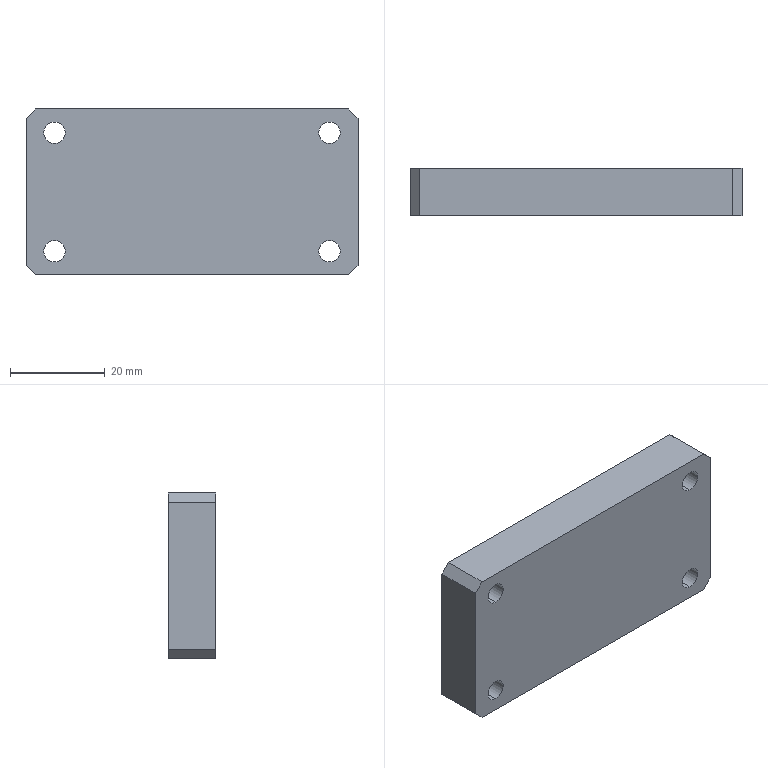Part | SolidWorks | features Chamfer 1, Extrusion 1, HoleWzd 1 | 1 solid | 30 faces | box 70 x 10 x 35 mm | volume 23097 mm3 | cylinder 16 | plane 14 | commonest cylinder face diameters 4.5 x8 8 x8
STEP:
#1=CARTESIAN_POINT('',(-29.,0.,-16.5));
#2=VERTEX_POINT('',#1);
#3=CARTESIAN_POINT('',(-29.,0.,-8.5));
#4=VERTEX_POINT('',#3);
#5=CARTESIAN_POINT('',(-29.,0.,-12.5));
#6=DIRECTION('',(0.,1.,0.));
#7=DIRECTION('',(0.,0.,1.));
#8=AXIS2_PLACEMENT_3D('',#5,#6,#7);
#9=CIRCLE('',#8,4.);
#10=EDGE_CURVE('',#2,#4,#9,.T.);
#11=ORIENTED_EDGE('',*,*,#10,.F.);
#12=CARTESIAN_POINT('',(-29.,5.,-16.5));
#13=VERTEX_POINT('',#12);
#14=CARTESIAN_POINT('',(-29.,5.,-16.5));
#15=DIRECTION('',(0.,1.,0.));
#16=VECTOR('',#15,1000.);
#17=LINE('',#14,#16);
#18=EDGE_CURVE('',#2,#13,#17,.T.);
#19=ORIENTED_EDGE('',*,*,#18,.T.);
#20=CARTESIAN_POINT('',(-29.,5.,-8.5));
#21=VERTEX_POINT('',#20);
#22=CARTESIAN_POINT('',(-29.,5.,-12.5));
#23=DIRECTION('',(0.,1.,0.));
#24=DIRECTION('',(0.,0.,1.));
#25=AXIS2_PLACEMENT_3D('',#22,#23,#24);
#26=CIRCLE('',#25,4.);
#27=EDGE_CURVE('',#13,#21,#26,.T.);
#28=ORIENTED_EDGE('',*,*,#27,.T.);
#29=CARTESIAN_POINT('',(-29.,5.,-8.5));
#30=DIRECTION('',(0.,1.,0.));
#31=VECTOR('',#30,1000.);
#32=LINE('',#29,#31);
#33=EDGE_CURVE('',#4,#21,#32,.T.);
#34=ORIENTED_EDGE('',*,*,#33,.F.);
#35=EDGE_LOOP('',(#11,#19,#28,#34));
#36=FACE_OUTER_BOUND('',#35,.T.);
#37=CARTESIAN_POINT('',(-29.,5.,-12.5));
#38=DIRECTION('',(0.,1.,0.));
#39=DIRECTION('',(0.,0.,1.));
#40=AXIS2_PLACEMENT_3D('',#37,#38,#39);
#41=CYLINDRICAL_SURFACE('',#40,4.);
#42=ADVANCED_FACE('',(#36),#41,.F.);
#43=CARTESIAN_POINT('',(-29.,-5.,-10.25));
#44=VERTEX_POINT('',#43);
#45=CARTESIAN_POINT('',(-29.,-5.,-14.75));
#46=VERTEX_POINT('',#45);
#47=CARTESIAN_POINT('',(-29.,-5.,-12.5));
#48=DIRECTION('',(0.,-1.,0.));
#49=DIRECTION('',(0.,0.,-1.));
#50=AXIS2_PLACEMENT_3D('',#47,#48,#49);
#51=CIRCLE('',#50,2.25);
#52=EDGE_CURVE('',#44,#46,#51,.T.);
#53=ORIENTED_EDGE('',*,*,#52,.T.);
#54=CARTESIAN_POINT('',(-29.,0.,-14.75));
#55=VERTEX_POINT('',#54);
#56=CARTESIAN_POINT('',(-29.,5.,-14.75));
#57=DIRECTION('',(0.,1.,0.));
#58=VECTOR('',#57,1000.);
#59=LINE('',#56,#58);
#60=EDGE_CURVE('',#46,#55,#59,.T.);
#61=ORIENTED_EDGE('',*,*,#60,.T.);
#62=CARTESIAN_POINT('',(-29.,0.,-10.25));
#63=VERTEX_POINT('',#62);
#64=CARTESIAN_POINT('',(-29.,0.,-12.5));
#65=DIRECTION('',(0.,1.,0.));
#66=DIRECTION('',(0.,0.,1.));
#67=AXIS2_PLACEMENT_3D('',#64,#65,#66);
#68=CIRCLE('',#67,2.25);
#69=EDGE_CURVE('',#55,#63,#68,.T.);
#70=ORIENTED_EDGE('',*,*,#69,.T.);
#71=CARTESIAN_POINT('',(-29.,5.,-10.25));
#72=DIRECTION('',(0.,1.,0.));
#73=VECTOR('',#72,1000.);
#74=LINE('',#71,#73);
#75=EDGE_CURVE('',#44,#63,#74,.T.);
#76=ORIENTED_EDGE('',*,*,#75,.F.);
#77=EDGE_LOOP('',(#53,#61,#70,#76));
#78=FACE_OUTER_BOUND('',#77,.T.);
#79=CARTESIAN_POINT('',(-29.,5.,-12.5));
#80=DIRECTION('',(0.,1.,0.));
#81=DIRECTION('',(0.,0.,1.));
#82=AXIS2_PLACEMENT_3D('',#79,#80,#81);
#83=CYLINDRICAL_SURFACE('',#82,2.25);
#84=ADVANCED_FACE('',(#78),#83,.F.);
#85=CARTESIAN_POINT('',(-29.,0.,8.5));
#86=VERTEX_POINT('',#85);
#87=CARTESIAN_POINT('',(-29.,0.,16.5));
#88=VERTEX_POINT('',#87);
#89=CARTESIAN_POINT('',(-29.,0.,12.5));
#90=DIRECTION('',(0.,1.,0.));
#91=DIRECTION('',(0.,0.,1.));
#92=AXIS2_PLACEMENT_3D('',#89,#90,#91);
#93=CIRCLE('',#92,4.);
#94=EDGE_CURVE('',#86,#88,#93,.T.);
#95=ORIENTED_EDGE('',*,*,#94,.F.);
#96=CARTESIAN_POINT('',(-29.,5.,8.5));
#97=VERTEX_POINT('',#96);
#98=CARTESIAN_POINT('',(-29.,5.,8.5));
#99=DIRECTION('',(0.,1.,0.));
#100=VECTOR('',#99,1000.);
#101=LINE('',#98,#100);
#102=EDGE_CURVE('',#86,#97,#101,.T.);
#103=ORIENTED_EDGE('',*,*,#102,.T.);
#104=CARTESIAN_POINT('',(-29.,5.,16.5));
#105=VERTEX_POINT('',#104);
#106=CARTESIAN_POINT('',(-29.,5.,12.5));
#107=DIRECTION('',(0.,1.,0.));
#108=DIRECTION('',(0.,0.,1.));
#109=AXIS2_PLACEMENT_3D('',#106,#107,#108);
#110=CIRCLE('',#109,4.);
#111=EDGE_CURVE('',#97,#105,#110,.T.);
#112=ORIENTED_EDGE('',*,*,#111,.T.);
#113=CARTESIAN_POINT('',(-29.,5.,16.5));
#114=DIRECTION('',(0.,1.,0.));
#115=VECTOR('',#114,1000.);
#116=LINE('',#113,#115);
#117=EDGE_CURVE('',#88,#105,#116,.T.);
#118=ORIENTED_EDGE('',*,*,#117,.F.);
#119=EDGE_LOOP('',(#95,#103,#112,#118));
#120=FACE_OUTER_BOUND('',#119,.T.);
#121=CARTESIAN_POINT('',(-29.,5.,12.5));
#122=DIRECTION('',(0.,1.,0.));
#123=DIRECTION('',(0.,0.,1.));
#124=AXIS2_PLACEMENT_3D('',#121,#122,#123);
#125=CYLINDRICAL_SURFACE('',#124,4.);
#126=ADVANCED_FACE('',(#120),#125,.F.);
#127=CARTESIAN_POINT('',(-29.,-5.,14.75));
#128=VERTEX_POINT('',#127);
#129=CARTESIAN_POINT('',(-29.,-5.,10.25));
#130=VERTEX_POINT('',#129);
#131=CARTESIAN_POINT('',(-29.,-5.,12.5));
#132=DIRECTION('',(0.,-1.,0.));
#133=DIRECTION('',(0.,0.,-1.));
#134=AXIS2_PLACEMENT_3D('',#131,#132,#133);
#135=CIRCLE('',#134,2.25);
#136=EDGE_CURVE('',#128,#130,#135,.T.);
#137=ORIENTED_EDGE('',*,*,#136,.T.);
#138=CARTESIAN_POINT('',(-29.,0.,10.25));
#139=VERTEX_POINT('',#138);
#140=CARTESIAN_POINT('',(-29.,5.,10.25));
#141=DIRECTION('',(0.,1.,0.));
#142=VECTOR('',#141,1000.);
#143=LINE('',#140,#142);
#144=EDGE_CURVE('',#130,#139,#143,.T.);
#145=ORIENTED_EDGE('',*,*,#144,.T.);
#146=CARTESIAN_POINT('',(-29.,0.,14.75));
#147=VERTEX_POINT('',#146);
#148=CARTESIAN_POINT('',(-29.,0.,12.5));
#149=DIRECTION('',(0.,1.,0.));
#150=DIRECTION('',(0.,0.,1.));
#151=AXIS2_PLACEMENT_3D('',#148,#149,#150);
#152=CIRCLE('',#151,2.25);
#153=EDGE_CURVE('',#139,#147,#152,.T.);
#154=ORIENTED_EDGE('',*,*,#153,.T.);
#155=CARTESIAN_POINT('',(-29.,5.,14.75));
#156=DIRECTION('',(0.,1.,0.));
#157=VECTOR('',#156,1000.);
#158=LINE('',#155,#157);
#159=EDGE_CURVE('',#128,#147,#158,.T.);
#160=ORIENTED_EDGE('',*,*,#159,.F.);
#161=EDGE_LOOP('',(#137,#145,#154,#160));
#162=FACE_OUTER_BOUND('',#161,.T.);
#163=CARTESIAN_POINT('',(-29.,5.,12.5));
#164=DIRECTION('',(0.,1.,0.));
#165=DIRECTION('',(0.,0.,1.));
#166=AXIS2_PLACEMENT_3D('',#163,#164,#165);
#167=CYLINDRICAL_SURFACE('',#166,2.25);
#168=ADVANCED_FACE('',(#162),#167,.F.);
#169=CARTESIAN_POINT('',(29.,0.,-16.5));
#170=VERTEX_POINT('',#169);
#171=CARTESIAN_POINT('',(29.,0.,-8.5));
#172=VERTEX_POINT('',#171);
#173=CARTESIAN_POINT('',(29.,0.,-12.5));
#174=DIRECTION('',(0.,1.,0.));
#175=DIRECTION('',(0.,0.,1.));
#176=AXIS2_PLACEMENT_3D('',#173,#174,#175);
#177=CIRCLE('',#176,4.);
#178=EDGE_CURVE('',#170,#172,#177,.T.);
#179=ORIENTED_EDGE('',*,*,#178,.F.);
#180=CARTESIAN_POINT('',(29.,5.,-16.5));
#181=VERTEX_POINT('',#180);
#182=CARTESIAN_POINT('',(29.,5.,-16.5));
#183=DIRECTION('',(0.,1.,0.));
#184=VECTOR('',#183,1000.);
#185=LINE('',#182,#184);
#186=EDGE_CURVE('',#170,#181,#185,.T.);
#187=ORIENTED_EDGE('',*,*,#186,.T.);
#188=CARTESIAN_POINT('',(29.,5.,-8.5));
#189=VERTEX_POINT('',#188);
#190=CARTESIAN_POINT('',(29.,5.,-12.5));
#191=DIRECTION('',(0.,1.,0.));
#192=DIRECTION('',(0.,0.,1.));
#193=AXIS2_PLACEMENT_3D('',#190,#191,#192);
#194=CIRCLE('',#193,4.);
#195=EDGE_CURVE('',#181,#189,#194,.T.);
#196=ORIENTED_EDGE('',*,*,#195,.T.);
#197=CARTESIAN_POINT('',(29.,5.,-8.5));
#198=DIRECTION('',(0.,1.,0.));
#199=VECTOR('',#198,1000.);
#200=LINE('',#197,#199);
#201=EDGE_CURVE('',#172,#189,#200,.T.);
#202=ORIENTED_EDGE('',*,*,#201,.F.);
#203=EDGE_LOOP('',(#179,#187,#196,#202));
#204=FACE_OUTER_BOUND('',#203,.T.);
#205=CARTESIAN_POINT('',(29.,5.,-12.5));
#206=DIRECTION('',(0.,1.,0.));
#207=DIRECTION('',(0.,0.,1.));
#208=AXIS2_PLACEMENT_3D('',#205,#206,#207);
#209=CYLINDRICAL_SURFACE('',#208,4.);
#210=ADVANCED_FACE('',(#204),#209,.F.);
#211=CARTESIAN_POINT('',(29.,-5.,-10.25));
#212=VERTEX_POINT('',#211);
#213=CARTESIAN_POINT('',(29.,-5.,-14.75));
#214=VERTEX_POINT('',#213);
#215=CARTESIAN_POINT('',(29.,-5.,-12.5));
#216=DIRECTION('',(0.,-1.,0.));
#217=DIRECTION('',(0.,0.,-1.));
#218=AXIS2_PLACEMENT_3D('',#215,#216,#217);
#219=CIRCLE('',#218,2.25);
#220=EDGE_CURVE('',#212,#214,#219,.T.);
#221=ORIENTED_EDGE('',*,*,#220,.T.);
#222=CARTESIAN_POINT('',(29.,0.,-14.75));
#223=VERTEX_POINT('',#222);
#224=CARTESIAN_POINT('',(29.,5.,-14.75));
#225=DIRECTION('',(0.,1.,0.));
#226=VECTOR('',#225,1000.);
#227=LINE('',#224,#226);
#228=EDGE_CURVE('',#214,#223,#227,.T.);
#229=ORIENTED_EDGE('',*,*,#228,.T.);
#230=CARTESIAN_POINT('',(29.,0.,-10.25));
#231=VERTEX_POINT('',#230);
#232=CARTESIAN_POINT('',(29.,0.,-12.5));
#233=DIRECTION('',(0.,1.,0.));
#234=DIRECTION('',(0.,0.,1.));
#235=AXIS2_PLACEMENT_3D('',#232,#233,#234);
#236=CIRCLE('',#235,2.25);
#237=EDGE_CURVE('',#223,#231,#236,.T.);
#238=ORIENTED_EDGE('',*,*,#237,.T.);
#239=CARTESIAN_POINT('',(29.,5.,-10.25));
#240=DIRECTION('',(0.,1.,0.));
#241=VECTOR('',#240,1000.);
#242=LINE('',#239,#241);
#243=EDGE_CURVE('',#212,#231,#242,.T.);
#244=ORIENTED_EDGE('',*,*,#243,.F.);
#245=EDGE_LOOP('',(#221,#229,#238,#244));
#246=FACE_OUTER_BOUND('',#245,.T.);
#247=CARTESIAN_POINT('',(29.,5.,-12.5));
#248=DIRECTION('',(0.,1.,0.));
#249=DIRECTION('',(0.,0.,1.));
#250=AXIS2_PLACEMENT_3D('',#247,#248,#249);
#251=CYLINDRICAL_SURFACE('',#250,2.25);
#252=ADVANCED_FACE('',(#246),#251,.F.);
#253=CARTESIAN_POINT('',(29.,0.,8.5));
#254=VERTEX_POINT('',#253);
#255=CARTESIAN_POINT('',(29.,0.,16.5));
#256=VERTEX_POINT('',#255);
#257=CARTESIAN_POINT('',(29.,0.,12.5));
#258=DIRECTION('',(0.,1.,0.));
#259=DIRECTION('',(0.,0.,1.));
#260=AXIS2_PLACEMENT_3D('',#257,#258,#259);
#261=CIRCLE('',#260,4.);
#262=EDGE_CURVE('',#254,#256,#261,.T.);
#263=ORIENTED_EDGE('',*,*,#262,.F.);
#264=CARTESIAN_POINT('',(29.,5.,8.5));
#265=VERTEX_POINT('',#264);
#266=CARTESIAN_POINT('',(29.,5.,8.5));
#267=DIRECTION('',(0.,1.,0.));
#268=VECTOR('',#267,1000.);
#269=LINE('',#266,#268);
#270=EDGE_CURVE('',#254,#265,#269,.T.);
#271=ORIENTED_EDGE('',*,*,#270,.T.);
#272=CARTESIAN_POINT('',(29.,5.,16.5));
#273=VERTEX_POINT('',#272);
#274=CARTESIAN_POINT('',(29.,5.,12.5));
#275=DIRECTION('',(0.,1.,0.));
#276=DIRECTION('',(0.,0.,1.));
#277=AXIS2_PLACEMENT_3D('',#274,#275,#276);
#278=CIRCLE('',#277,4.);
#279=EDGE_CURVE('',#265,#273,#278,.T.);
#280=ORIENTED_EDGE('',*,*,#279,.T.);
#281=CARTESIAN_POINT('',(29.,5.,16.5));
#282=DIRECTION('',(0.,1.,0.));
#283=VECTOR('',#282,1000.);
#284=LINE('',#281,#283);
#285=EDGE_CURVE('',#256,#273,#284,.T.);
#286=ORIENTED_EDGE('',*,*,#285,.F.);
#287=EDGE_LOOP('',(#263,#271,#280,#286));
#288=FACE_OUTER_BOUND('',#287,.T.);
#289=CARTESIAN_POINT('',(29.,5.,12.5));
#290=DIRECTION('',(0.,1.,0.));
#291=DIRECTION('',(0.,0.,1.));
#292=AXIS2_PLACEMENT_3D('',#289,#290,#291);
#293=CYLINDRICAL_SURFACE('',#292,4.);
#294=ADVANCED_FACE('',(#288),#293,.F.);
#295=CARTESIAN_POINT('',(29.,-5.,14.75));
#296=VERTEX_POINT('',#295);
#297=CARTESIAN_POINT('',(29.,-5.,10.25));
#298=VERTEX_POINT('',#297);
#299=CARTESIAN_POINT('',(29.,-5.,12.5));
#300=DIRECTION('',(0.,-1.,0.));
#301=DIRECTION('',(0.,0.,-1.));
#302=AXIS2_PLACEMENT_3D('',#299,#300,#301);
#303=CIRCLE('',#302,2.25);
#304=EDGE_CURVE('',#296,#298,#303,.T.);
#305=ORIENTED_EDGE('',*,*,#304,.T.);
#306=CARTESIAN_POINT('',(29.,0.,10.25));
#307=VERTEX_POINT('',#306);
#308=CARTESIAN_POINT('',(29.,5.,10.25));
#309=DIRECTION('',(0.,1.,0.));
#310=VECTOR('',#309,1000.);
#311=LINE('',#308,#310);
#312=EDGE_CURVE('',#298,#307,#311,.T.);
#313=ORIENTED_EDGE('',*,*,#312,.T.);
#314=CARTESIAN_POINT('',(29.,0.,14.75));
#315=VERTEX_POINT('',#314);
#316=CARTESIAN_POINT('',(29.,0.,12.5));
#317=DIRECTION('',(0.,1.,0.));
#318=DIRECTION('',(0.,0.,1.));
#319=AXIS2_PLACEMENT_3D('',#316,#317,#318);
#320=CIRCLE('',#319,2.25);
#321=EDGE_CURVE('',#307,#315,#320,.T.);
#322=ORIENTED_EDGE('',*,*,#321,.T.);
#323=CARTESIAN_POINT('',(29.,5.,14.75));
#324=DIRECTION('',(0.,1.,0.));
#325=VECTOR('',#324,1000.);
#326=LINE('',#323,#325);
#327=EDGE_CURVE('',#296,#315,#326,.T.);
#328=ORIENTED_EDGE('',*,*,#327,.F.);
#329=EDGE_LOOP('',(#305,#313,#322,#328));
#330=FACE_OUTER_BOUND('',#329,.T.);
#331=CARTESIAN_POINT('',(29.,5.,12.5));
#332=DIRECTION('',(0.,1.,0.));
#333=DIRECTION('',(0.,0.,1.));
#334=AXIS2_PLACEMENT_3D('',#331,#332,#333);
#335=CYLINDRICAL_SURFACE('',#334,2.25);
#336=ADVANCED_FACE('',(#330),#335,.F.);
#337=CARTESIAN_POINT('',(-29.,5.,-12.5));
#338=DIRECTION('',(0.,1.,0.));
#339=DIRECTION('',(0.,0.,1.));
#340=AXIS2_PLACEMENT_3D('',#337,#338,#339);
#341=CIRCLE('',#340,4.);
#342=EDGE_CURVE('',#21,#13,#341,.T.);
#343=ORIENTED_EDGE('',*,*,#342,.F.);
#344=ORIENTED_EDGE('',*,*,#27,.F.);
#345=EDGE_LOOP('',(#343,#344));
#346=FACE_BOUND('',#345,.T.);
#347=CARTESIAN_POINT('',(29.,5.,12.5));
#348=DIRECTION('',(0.,1.,0.));
#349=DIRECTION('',(0.,0.,1.));
#350=AXIS2_PLACEMENT_3D('',#347,#348,#349);
#351=CIRCLE('',#350,4.);
#352=EDGE_CURVE('',#273,#265,#351,.T.);
#353=ORIENTED_EDGE('',*,*,#352,.F.);
#354=ORIENTED_EDGE('',*,*,#279,.F.);
#355=EDGE_LOOP('',(#353,#354));
#356=FACE_BOUND('',#355,.T.);
#357=CARTESIAN_POINT('',(33.,5.,-17.5));
#358=VERTEX_POINT('',#357);
#359=CARTESIAN_POINT('',(-33.,5.,-17.5));
#360=VERTEX_POINT('',#359);
#361=CARTESIAN_POINT('',(-35.,5.,-17.5));
#362=DIRECTION('',(-1.,0.,0.));
#363=VECTOR('',#362,1000.);
#364=LINE('',#361,#363);
#365=EDGE_CURVE('',#358,#360,#364,.T.);
#366=ORIENTED_EDGE('',*,*,#365,.T.);
#367=CARTESIAN_POINT('',(-35.,5.,-15.5));
#368=VERTEX_POINT('',#367);
#369=CARTESIAN_POINT('',(-35.,5.,-15.5));
#370=DIRECTION('',(-0.7071,0.,0.7071));
#371=VECTOR('',#370,1000.);
#372=LINE('',#369,#371);
#373=EDGE_CURVE('',#360,#368,#372,.T.);
#374=ORIENTED_EDGE('',*,*,#373,.T.);
#375=CARTESIAN_POINT('',(-35.,5.,15.5));
#376=VERTEX_POINT('',#375);
#377=CARTESIAN_POINT('',(-35.,5.,17.5));
#378=DIRECTION('',(0.,0.,1.));
#379=VECTOR('',#378,1000.);
#380=LINE('',#377,#379);
#381=EDGE_CURVE('',#368,#376,#380,.T.);
#382=ORIENTED_EDGE('',*,*,#381,.T.);
#383=CARTESIAN_POINT('',(-33.,5.,17.5));
#384=VERTEX_POINT('',#383);
#385=CARTESIAN_POINT('',(-33.,5.,17.5));
#386=DIRECTION('',(0.7071,0.,0.7071));
#387=VECTOR('',#386,1000.);
#388=LINE('',#385,#387);
#389=EDGE_CURVE('',#376,#384,#388,.T.);
#390=ORIENTED_EDGE('',*,*,#389,.T.);
#391=CARTESIAN_POINT('',(33.,5.,17.5));
#392=VERTEX_POINT('',#391);
#393=CARTESIAN_POINT('',(-35.,5.,17.5));
#394=DIRECTION('',(1.,0.,0.));
#395=VECTOR('',#394,1000.);
#396=LINE('',#393,#395);
#397=EDGE_CURVE('',#384,#392,#396,.T.);
#398=ORIENTED_EDGE('',*,*,#397,.T.);
#399=CARTESIAN_POINT('',(35.,5.,15.5));
#400=VERTEX_POINT('',#399);
#401=CARTESIAN_POINT('',(35.,5.,15.5));
#402=DIRECTION('',(0.7071,0.,-0.7071));
#403=VECTOR('',#402,1000.);
#404=LINE('',#401,#403);
#405=EDGE_CURVE('',#392,#400,#404,.T.);
#406=ORIENTED_EDGE('',*,*,#405,.T.);
#407=CARTESIAN_POINT('',(35.,5.,-15.5));
#408=VERTEX_POINT('',#407);
#409=CARTESIAN_POINT('',(35.,5.,17.5));
#410=DIRECTION('',(0.,0.,-1.));
#411=VECTOR('',#410,1000.);
#412=LINE('',#409,#411);
#413=EDGE_CURVE('',#400,#408,#412,.T.);
#414=ORIENTED_EDGE('',*,*,#413,.T.);
#415=CARTESIAN_POINT('',(33.,5.,-17.5));
#416=DIRECTION('',(-0.7071,0.,-0.7071));
#417=VECTOR('',#416,1000.);
#418=LINE('',#415,#417);
#419=EDGE_CURVE('',#408,#358,#418,.T.);
#420=ORIENTED_EDGE('',*,*,#419,.T.);
#421=EDGE_LOOP('',(#366,#374,#382,#390,#398,#406,#414,#420));
#422=FACE_OUTER_BOUND('',#421,.T.);
#423=CARTESIAN_POINT('',(29.,5.,-12.5));
#424=DIRECTION('',(0.,1.,0.));
#425=DIRECTION('',(0.,0.,1.));
#426=AXIS2_PLACEMENT_3D('',#423,#424,#425);
#427=CIRCLE('',#426,4.);
#428=EDGE_CURVE('',#189,#181,#427,.T.);
#429=ORIENTED_EDGE('',*,*,#428,.F.);
#430=ORIENTED_EDGE('',*,*,#195,.F.);
#431=EDGE_LOOP('',(#429,#430));
#432=FACE_BOUND('',#431,.T.);
#433=CARTESIAN_POINT('',(-29.,5.,12.5));
#434=DIRECTION('',(0.,1.,0.));
#435=DIRECTION('',(0.,0.,1.));
#436=AXIS2_PLACEMENT_3D('',#433,#434,#435);
#437=CIRCLE('',#436,4.);
#438=EDGE_CURVE('',#105,#97,#437,.T.);
#439=ORIENTED_EDGE('',*,*,#438,.F.);
#440=ORIENTED_EDGE('',*,*,#111,.F.);
#441=EDGE_LOOP('',(#439,#440));
#442=FACE_BOUND('',#441,.T.);
#443=CARTESIAN_POINT('',(0.,5.,0.));
#444=DIRECTION('',(0.,-1.,0.));
#445=DIRECTION('',(0.,0.,-1.));
#446=AXIS2_PLACEMENT_3D('',#443,#444,#445);
#447=PLANE('',#446);
#448=ADVANCED_FACE('',(#346,#356,#422,#432,#442),#447,.F.);
#449=CARTESIAN_POINT('',(35.,-5.,15.5));
#450=VERTEX_POINT('',#449);
#451=CARTESIAN_POINT('',(35.,-5.,-15.5));
#452=VERTEX_POINT('',#451);
#453=CARTESIAN_POINT('',(35.,-5.,17.5));
#454=DIRECTION('',(0.,0.,-1.));
#455=VECTOR('',#454,1000.);
#456=LINE('',#453,#455);
#457=EDGE_CURVE('',#450,#452,#456,.T.);
#458=ORIENTED_EDGE('',*,*,#457,.T.);
#459=CARTESIAN_POINT('',(35.,5.,-15.5));
#460=DIRECTION('',(0.,1.,0.));
#461=VECTOR('',#460,1000.);
#462=LINE('',#459,#461);
#463=EDGE_CURVE('',#452,#408,#462,.T.);
#464=ORIENTED_EDGE('',*,*,#463,.T.);
#465=ORIENTED_EDGE('',*,*,#413,.F.);
#466=CARTESIAN_POINT('',(35.,5.,15.5));
#467=DIRECTION('',(0.,-1.,0.));
#468=VECTOR('',#467,1000.);
#469=LINE('',#466,#468);
#470=EDGE_CURVE('',#400,#450,#469,.T.);
#471=ORIENTED_EDGE('',*,*,#470,.T.);
#472=EDGE_LOOP('',(#458,#464,#465,#471));
#473=FACE_OUTER_BOUND('',#472,.T.);
#474=CARTESIAN_POINT('',(35.,5.,17.5));
#475=DIRECTION('',(-1.,0.,0.));
#476=DIRECTION('',(0.,0.,1.));
#477=AXIS2_PLACEMENT_3D('',#474,#475,#476);
#478=PLANE('',#477);
#479=ADVANCED_FACE('',(#473),#478,.F.);
#480=CARTESIAN_POINT('',(33.,-5.,-17.5));
#481=VERTEX_POINT('',#480);
#482=CARTESIAN_POINT('',(-33.,-5.,-17.5));
#483=VERTEX_POINT('',#482);
#484=CARTESIAN_POINT('',(-35.,-5.,-17.5));
#485=DIRECTION('',(-1.,0.,0.));
#486=VECTOR('',#485,1000.);
#487=LINE('',#484,#486);
#488=EDGE_CURVE('',#481,#483,#487,.T.);
#489=ORIENTED_EDGE('',*,*,#488,.T.);
#490=CARTESIAN_POINT('',(-33.,5.,-17.5));
#491=DIRECTION('',(0.,1.,0.));
#492=VECTOR('',#491,1000.);
#493=LINE('',#490,#492);
#494=EDGE_CURVE('',#483,#360,#493,.T.);
#495=ORIENTED_EDGE('',*,*,#494,.T.);
#496=ORIENTED_EDGE('',*,*,#365,.F.);
#497=CARTESIAN_POINT('',(33.,5.,-17.5));
#498=DIRECTION('',(0.,-1.,0.));
#499=VECTOR('',#498,1000.);
#500=LINE('',#497,#499);
#501=EDGE_CURVE('',#358,#481,#500,.T.);
#502=ORIENTED_EDGE('',*,*,#501,.T.);
#503=EDGE_LOOP('',(#489,#495,#496,#502));
#504=FACE_OUTER_BOUND('',#503,.T.);
#505=CARTESIAN_POINT('',(-35.,5.,-17.5));
#506=DIRECTION('',(0.,0.,1.));
#507=DIRECTION('',(1.,0.,0.));
#508=AXIS2_PLACEMENT_3D('',#505,#506,#507);
#509=PLANE('',#508);
#510=ADVANCED_FACE('',(#504),#509,.F.);
#511=ORIENTED_EDGE('',*,*,#381,.F.);
#512=CARTESIAN_POINT('',(-35.,-5.,-15.5));
#513=VERTEX_POINT('',#512);
#514=CARTESIAN_POINT('',(-35.,5.,-15.5));
#515=DIRECTION('',(0.,-1.,0.));
#516=VECTOR('',#515,1000.);
#517=LINE('',#514,#516);
#518=EDGE_CURVE('',#368,#513,#517,.T.);
#519=ORIENTED_EDGE('',*,*,#518,.T.);
#520=CARTESIAN_POINT('',(-35.,-5.,15.5));
#521=VERTEX_POINT('',#520);
#522=CARTESIAN_POINT('',(-35.,-5.,17.5));
#523=DIRECTION('',(0.,0.,1.));
#524=VECTOR('',#523,1000.);
#525=LINE('',#522,#524);
#526=EDGE_CURVE('',#513,#521,#525,.T.);
#527=ORIENTED_EDGE('',*,*,#526,.T.);
#528=CARTESIAN_POINT('',(-35.,5.,15.5));
#529=DIRECTION('',(0.,1.,0.));
#530=VECTOR('',#529,1000.);
#531=LINE('',#528,#530);
#532=EDGE_CURVE('',#521,#376,#531,.T.);
#533=ORIENTED_EDGE('',*,*,#532,.T.);
#534=EDGE_LOOP('',(#511,#519,#527,#533));
#535=FACE_OUTER_BOUND('',#534,.T.);
#536=CARTESIAN_POINT('',(-35.,5.,17.5));
#537=DIRECTION('',(1.,0.,0.));
#538=DIRECTION('',(0.,0.,-1.));
#539=AXIS2_PLACEMENT_3D('',#536,#537,#538);
#540=PLANE('',#539);
#541=ADVANCED_FACE('',(#535),#540,.F.);
#542=CARTESIAN_POINT('',(-33.,-5.,17.5));
#543=VERTEX_POINT('',#542);
#544=CARTESIAN_POINT('',(33.,-5.,17.5));
#545=VERTEX_POINT('',#544);
#546=CARTESIAN_POINT('',(-35.,-5.,17.5));
#547=DIRECTION('',(1.,0.,0.));
#548=VECTOR('',#547,1000.);
#549=LINE('',#546,#548);
#550=EDGE_CURVE('',#543,#545,#549,.T.);
#551=ORIENTED_EDGE('',*,*,#550,.T.);
#552=CARTESIAN_POINT('',(33.,5.,17.5));
#553=DIRECTION('',(0.,1.,0.));
#554=VECTOR('',#553,1000.);
#555=LINE('',#552,#554);
#556=EDGE_CURVE('',#545,#392,#555,.T.);
#557=ORIENTED_EDGE('',*,*,#556,.T.);
#558=ORIENTED_EDGE('',*,*,#397,.F.);
#559=CARTESIAN_POINT('',(-33.,5.,17.5));
#560=DIRECTION('',(0.,-1.,0.));
#561=VECTOR('',#560,1000.);
#562=LINE('',#559,#561);
#563=EDGE_CURVE('',#384,#543,#562,.T.);
#564=ORIENTED_EDGE('',*,*,#563,.T.);
#565=EDGE_LOOP('',(#551,#557,#558,#564));
#566=FACE_OUTER_BOUND('',#565,.T.);
#567=CARTESIAN_POINT('',(-35.,5.,17.5));
#568=DIRECTION('',(0.,0.,-1.));
#569=DIRECTION('',(-1.,0.,0.));
#570=AXIS2_PLACEMENT_3D('',#567,#568,#569);
#571=PLANE('',#570);
#572=ADVANCED_FACE('',(#566),#571,.F.);
#573=ORIENTED_EDGE('',*,*,#52,.F.);
#574=CARTESIAN_POINT('',(-29.,-5.,-12.5));
#575=DIRECTION('',(0.,-1.,0.));
#576=DIRECTION('',(0.,0.,-1.));
#577=AXIS2_PLACEMENT_3D('',#574,#575,#576);
#578=CIRCLE('',#577,2.25);
#579=EDGE_CURVE('',#46,#44,#578,.T.);
#580=ORIENTED_EDGE('',*,*,#579,.F.);
#581=EDGE_LOOP('',(#573,#580));
#582=FACE_BOUND('',#581,.T.);
#583=ORIENTED_EDGE('',*,*,#136,.F.);
#584=CARTESIAN_POINT('',(-29.,-5.,12.5));
#585=DIRECTION('',(0.,-1.,0.));
#586=DIRECTION('',(0.,0.,-1.));
#587=AXIS2_PLACEMENT_3D('',#584,#585,#586);
#588=CIRCLE('',#587,2.25);
#589=EDGE_CURVE('',#130,#128,#588,.T.);
#590=ORIENTED_EDGE('',*,*,#589,.F.);
#591=EDGE_LOOP('',(#583,#590));
#592=FACE_BOUND('',#591,.T.);
#593=ORIENTED_EDGE('',*,*,#220,.F.);
#594=CARTESIAN_POINT('',(29.,-5.,-12.5));
#595=DIRECTION('',(0.,-1.,0.));
#596=DIRECTION('',(0.,0.,-1.));
#597=AXIS2_PLACEMENT_3D('',#594,#595,#596);
#598=CIRCLE('',#597,2.25);
#599=EDGE_CURVE('',#214,#212,#598,.T.);
#600=ORIENTED_EDGE('',*,*,#599,.F.);
#601=EDGE_LOOP('',(#593,#600));
#602=FACE_BOUND('',#601,.T.);
#603=ORIENTED_EDGE('',*,*,#304,.F.);
#604=CARTESIAN_POINT('',(29.,-5.,12.5));
#605=DIRECTION('',(0.,-1.,0.));
#606=DIRECTION('',(0.,0.,-1.));
#607=AXIS2_PLACEMENT_3D('',#604,#605,#606);
#608=CIRCLE('',#607,2.25);
#609=EDGE_CURVE('',#298,#296,#608,.T.);
#610=ORIENTED_EDGE('',*,*,#609,.F.);
#611=EDGE_LOOP('',(#603,#610));
#612=FACE_BOUND('',#611,.T.);
#613=ORIENTED_EDGE('',*,*,#526,.F.);
#614=CARTESIAN_POINT('',(-25.25,-5.,-25.25));
#615=DIRECTION('',(0.7071,0.,-0.7071));
#616=VECTOR('',#615,1000.);
#617=LINE('',#614,#616);
#618=EDGE_CURVE('',#513,#483,#617,.T.);
#619=ORIENTED_EDGE('',*,*,#618,.T.);
#620=ORIENTED_EDGE('',*,*,#488,.F.);
#621=CARTESIAN_POINT('',(25.25,-5.,-25.25));
#622=DIRECTION('',(0.7071,0.,0.7071));
#623=VECTOR('',#622,1000.);
#624=LINE('',#621,#623);
#625=EDGE_CURVE('',#481,#452,#624,.T.);
#626=ORIENTED_EDGE('',*,*,#625,.T.);
#627=ORIENTED_EDGE('',*,*,#457,.F.);
#628=CARTESIAN_POINT('',(25.25,-5.,25.25));
#629=DIRECTION('',(-0.7071,0.,0.7071));
#630=VECTOR('',#629,1000.);
#631=LINE('',#628,#630);
#632=EDGE_CURVE('',#450,#545,#631,.T.);
#633=ORIENTED_EDGE('',*,*,#632,.T.);
#634=ORIENTED_EDGE('',*,*,#550,.F.);
#635=CARTESIAN_POINT('',(-25.25,-5.,25.25));
#636=DIRECTION('',(-0.7071,0.,-0.7071));
#637=VECTOR('',#636,1000.);
#638=LINE('',#635,#637);
#639=EDGE_CURVE('',#543,#521,#638,.T.);
#640=ORIENTED_EDGE('',*,*,#639,.T.);
#641=EDGE_LOOP('',(#613,#619,#620,#626,#627,#633,#634,#640));
#642=FACE_OUTER_BOUND('',#641,.T.);
#643=CARTESIAN_POINT('',(0.,-5.,0.));
#644=DIRECTION('',(0.,-1.,0.));
#645=DIRECTION('',(0.,0.,-1.));
#646=AXIS2_PLACEMENT_3D('',#643,#644,#645);
#647=PLANE('',#646);
#648=ADVANCED_FACE('',(#582,#592,#602,#612,#642),#647,.T.);
#649=ORIENTED_EDGE('',*,*,#373,.F.);
#650=ORIENTED_EDGE('',*,*,#494,.F.);
#651=ORIENTED_EDGE('',*,*,#618,.F.);
#652=ORIENTED_EDGE('',*,*,#518,.F.);
#653=EDGE_LOOP('',(#649,#650,#651,#652));
#654=FACE_OUTER_BOUND('',#653,.T.);
#655=CARTESIAN_POINT('',(-35.,5.,-15.5));
#656=DIRECTION('',(0.7071,0.,0.7071));
#657=DIRECTION('',(0.,-1.,0.));
#658=AXIS2_PLACEMENT_3D('',#655,#656,#657);
#659=PLANE('',#658);
#660=ADVANCED_FACE('',(#654),#659,.F.);
#661=ORIENTED_EDGE('',*,*,#419,.F.);
#662=ORIENTED_EDGE('',*,*,#463,.F.);
#663=ORIENTED_EDGE('',*,*,#625,.F.);
#664=ORIENTED_EDGE('',*,*,#501,.F.);
#665=EDGE_LOOP('',(#661,#662,#663,#664));
#666=FACE_OUTER_BOUND('',#665,.T.);
#667=CARTESIAN_POINT('',(33.,5.,-17.5));
#668=DIRECTION('',(-0.7071,0.,0.7071));
#669=DIRECTION('',(0.,-1.,0.));
#670=AXIS2_PLACEMENT_3D('',#667,#668,#669);
#671=PLANE('',#670);
#672=ADVANCED_FACE('',(#666),#671,.F.);
#673=ORIENTED_EDGE('',*,*,#405,.F.);
#674=ORIENTED_EDGE('',*,*,#556,.F.);
#675=ORIENTED_EDGE('',*,*,#632,.F.);
#676=ORIENTED_EDGE('',*,*,#470,.F.);
#677=EDGE_LOOP('',(#673,#674,#675,#676));
#678=FACE_OUTER_BOUND('',#677,.T.);
#679=CARTESIAN_POINT('',(35.,5.,15.5));
#680=DIRECTION('',(-0.7071,0.,-0.7071));
#681=DIRECTION('',(0.,-1.,0.));
#682=AXIS2_PLACEMENT_3D('',#679,#680,#681);
#683=PLANE('',#682);
#684=ADVANCED_FACE('',(#678),#683,.F.);
#685=ORIENTED_EDGE('',*,*,#389,.F.);
#686=ORIENTED_EDGE('',*,*,#532,.F.);
#687=ORIENTED_EDGE('',*,*,#639,.F.);
#688=ORIENTED_EDGE('',*,*,#563,.F.);
#689=EDGE_LOOP('',(#685,#686,#687,#688));
#690=FACE_OUTER_BOUND('',#689,.T.);
#691=CARTESIAN_POINT('',(-33.,5.,17.5));
#692=DIRECTION('',(0.7071,0.,-0.7071));
#693=DIRECTION('',(0.,-1.,0.));
#694=AXIS2_PLACEMENT_3D('',#691,#692,#693);
#695=PLANE('',#694);
#696=ADVANCED_FACE('',(#690),#695,.F.);
#697=ORIENTED_EDGE('',*,*,#312,.F.);
#698=ORIENTED_EDGE('',*,*,#609,.T.);
#699=ORIENTED_EDGE('',*,*,#327,.T.);
#700=CARTESIAN_POINT('',(29.,0.,12.5));
#701=DIRECTION('',(0.,1.,0.));
#702=DIRECTION('',(0.,0.,1.));
#703=AXIS2_PLACEMENT_3D('',#700,#701,#702);
#704=CIRCLE('',#703,2.25);
#705=EDGE_CURVE('',#315,#307,#704,.T.);
#706=ORIENTED_EDGE('',*,*,#705,.T.);
#707=EDGE_LOOP('',(#697,#698,#699,#706));
#708=FACE_OUTER_BOUND('',#707,.T.);
#709=CARTESIAN_POINT('',(29.,5.,12.5));
#710=DIRECTION('',(0.,1.,0.));
#711=DIRECTION('',(0.,0.,1.));
#712=AXIS2_PLACEMENT_3D('',#709,#710,#711);
#713=CYLINDRICAL_SURFACE('',#712,2.25);
#714=ADVANCED_FACE('',(#708),#713,.F.);
#715=ORIENTED_EDGE('',*,*,#705,.F.);
#716=ORIENTED_EDGE('',*,*,#321,.F.);
#717=EDGE_LOOP('',(#715,#716));
#718=FACE_BOUND('',#717,.T.);
#719=CARTESIAN_POINT('',(29.,0.,12.5));
#720=DIRECTION('',(0.,1.,0.));
#721=DIRECTION('',(0.,0.,1.));
#722=AXIS2_PLACEMENT_3D('',#719,#720,#721);
#723=CIRCLE('',#722,4.);
#724=EDGE_CURVE('',#256,#254,#723,.T.);
#725=ORIENTED_EDGE('',*,*,#724,.T.);
#726=ORIENTED_EDGE('',*,*,#262,.T.);
#727=EDGE_LOOP('',(#725,#726));
#728=FACE_OUTER_BOUND('',#727,.T.);
#729=CARTESIAN_POINT('',(31.25,0.,12.5));
#730=DIRECTION('',(0.,-1.,0.));
#731=DIRECTION('',(0.,0.,-1.));
#732=AXIS2_PLACEMENT_3D('',#729,#730,#731);
#733=PLANE('',#732);
#734=ADVANCED_FACE('',(#718,#728),#733,.F.);
#735=ORIENTED_EDGE('',*,*,#270,.F.);
#736=ORIENTED_EDGE('',*,*,#724,.F.);
#737=ORIENTED_EDGE('',*,*,#285,.T.);
#738=ORIENTED_EDGE('',*,*,#352,.T.);
#739=EDGE_LOOP('',(#735,#736,#737,#738));
#740=FACE_OUTER_BOUND('',#739,.T.);
#741=CARTESIAN_POINT('',(29.,5.,12.5));
#742=DIRECTION('',(0.,1.,0.));
#743=DIRECTION('',(0.,0.,1.));
#744=AXIS2_PLACEMENT_3D('',#741,#742,#743);
#745=CYLINDRICAL_SURFACE('',#744,4.);
#746=ADVANCED_FACE('',(#740),#745,.F.);
#747=ORIENTED_EDGE('',*,*,#228,.F.);
#748=ORIENTED_EDGE('',*,*,#599,.T.);
#749=ORIENTED_EDGE('',*,*,#243,.T.);
#750=CARTESIAN_POINT('',(29.,0.,-12.5));
#751=DIRECTION('',(0.,1.,0.));
#752=DIRECTION('',(0.,0.,1.));
#753=AXIS2_PLACEMENT_3D('',#750,#751,#752);
#754=CIRCLE('',#753,2.25);
#755=EDGE_CURVE('',#231,#223,#754,.T.);
#756=ORIENTED_EDGE('',*,*,#755,.T.);
#757=EDGE_LOOP('',(#747,#748,#749,#756));
#758=FACE_OUTER_BOUND('',#757,.T.);
#759=CARTESIAN_POINT('',(29.,5.,-12.5));
#760=DIRECTION('',(0.,1.,0.));
#761=DIRECTION('',(0.,0.,1.));
#762=AXIS2_PLACEMENT_3D('',#759,#760,#761);
#763=CYLINDRICAL_SURFACE('',#762,2.25);
#764=ADVANCED_FACE('',(#758),#763,.F.);
#765=ORIENTED_EDGE('',*,*,#755,.F.);
#766=ORIENTED_EDGE('',*,*,#237,.F.);
#767=EDGE_LOOP('',(#765,#766));
#768=FACE_BOUND('',#767,.T.);
#769=CARTESIAN_POINT('',(29.,0.,-12.5));
#770=DIRECTION('',(0.,1.,0.));
#771=DIRECTION('',(0.,0.,1.));
#772=AXIS2_PLACEMENT_3D('',#769,#770,#771);
#773=CIRCLE('',#772,4.);
#774=EDGE_CURVE('',#172,#170,#773,.T.);
#775=ORIENTED_EDGE('',*,*,#774,.T.);
#776=ORIENTED_EDGE('',*,*,#178,.T.);
#777=EDGE_LOOP('',(#775,#776));
#778=FACE_OUTER_BOUND('',#777,.T.);
#779=CARTESIAN_POINT('',(31.25,0.,-12.5));
#780=DIRECTION('',(0.,-1.,0.));
#781=DIRECTION('',(0.,0.,-1.));
#782=AXIS2_PLACEMENT_3D('',#779,#780,#781);
#783=PLANE('',#782);
#784=ADVANCED_FACE('',(#768,#778),#783,.F.);
#785=ORIENTED_EDGE('',*,*,#186,.F.);
#786=ORIENTED_EDGE('',*,*,#774,.F.);
#787=ORIENTED_EDGE('',*,*,#201,.T.);
#788=ORIENTED_EDGE('',*,*,#428,.T.);
#789=EDGE_LOOP('',(#785,#786,#787,#788));
#790=FACE_OUTER_BOUND('',#789,.T.);
#791=CARTESIAN_POINT('',(29.,5.,-12.5));
#792=DIRECTION('',(0.,1.,0.));
#793=DIRECTION('',(0.,0.,1.));
#794=AXIS2_PLACEMENT_3D('',#791,#792,#793);
#795=CYLINDRICAL_SURFACE('',#794,4.);
#796=ADVANCED_FACE('',(#790),#795,.F.);
#797=ORIENTED_EDGE('',*,*,#144,.F.);
#798=ORIENTED_EDGE('',*,*,#589,.T.);
#799=ORIENTED_EDGE('',*,*,#159,.T.);
#800=CARTESIAN_POINT('',(-29.,0.,12.5));
#801=DIRECTION('',(0.,1.,0.));
#802=DIRECTION('',(0.,0.,1.));
#803=AXIS2_PLACEMENT_3D('',#800,#801,#802);
#804=CIRCLE('',#803,2.25);
#805=EDGE_CURVE('',#147,#139,#804,.T.);
#806=ORIENTED_EDGE('',*,*,#805,.T.);
#807=EDGE_LOOP('',(#797,#798,#799,#806));
#808=FACE_OUTER_BOUND('',#807,.T.);
#809=CARTESIAN_POINT('',(-29.,5.,12.5));
#810=DIRECTION('',(0.,1.,0.));
#811=DIRECTION('',(0.,0.,1.));
#812=AXIS2_PLACEMENT_3D('',#809,#810,#811);
#813=CYLINDRICAL_SURFACE('',#812,2.25);
#814=ADVANCED_FACE('',(#808),#813,.F.);
#815=ORIENTED_EDGE('',*,*,#805,.F.);
#816=ORIENTED_EDGE('',*,*,#153,.F.);
#817=EDGE_LOOP('',(#815,#816));
#818=FACE_BOUND('',#817,.T.);
#819=CARTESIAN_POINT('',(-29.,0.,12.5));
#820=DIRECTION('',(0.,1.,0.));
#821=DIRECTION('',(0.,0.,1.));
#822=AXIS2_PLACEMENT_3D('',#819,#820,#821);
#823=CIRCLE('',#822,4.);
#824=EDGE_CURVE('',#88,#86,#823,.T.);
#825=ORIENTED_EDGE('',*,*,#824,.T.);
#826=ORIENTED_EDGE('',*,*,#94,.T.);
#827=EDGE_LOOP('',(#825,#826));
#828=FACE_OUTER_BOUND('',#827,.T.);
#829=CARTESIAN_POINT('',(-26.75,0.,12.5));
#830=DIRECTION('',(0.,-1.,0.));
#831=DIRECTION('',(0.,0.,-1.));
#832=AXIS2_PLACEMENT_3D('',#829,#830,#831);
#833=PLANE('',#832);
#834=ADVANCED_FACE('',(#818,#828),#833,.F.);
#835=ORIENTED_EDGE('',*,*,#102,.F.);
#836=ORIENTED_EDGE('',*,*,#824,.F.);
#837=ORIENTED_EDGE('',*,*,#117,.T.);
#838=ORIENTED_EDGE('',*,*,#438,.T.);
#839=EDGE_LOOP('',(#835,#836,#837,#838));
#840=FACE_OUTER_BOUND('',#839,.T.);
#841=CARTESIAN_POINT('',(-29.,5.,12.5));
#842=DIRECTION('',(0.,1.,0.));
#843=DIRECTION('',(0.,0.,1.));
#844=AXIS2_PLACEMENT_3D('',#841,#842,#843);
#845=CYLINDRICAL_SURFACE('',#844,4.);
#846=ADVANCED_FACE('',(#840),#845,.F.);
#847=ORIENTED_EDGE('',*,*,#60,.F.);
#848=ORIENTED_EDGE('',*,*,#579,.T.);
#849=ORIENTED_EDGE('',*,*,#75,.T.);
#850=CARTESIAN_POINT('',(-29.,0.,-12.5));
#851=DIRECTION('',(0.,1.,0.));
#852=DIRECTION('',(0.,0.,1.));
#853=AXIS2_PLACEMENT_3D('',#850,#851,#852);
#854=CIRCLE('',#853,2.25);
#855=EDGE_CURVE('',#63,#55,#854,.T.);
#856=ORIENTED_EDGE('',*,*,#855,.T.);
#857=EDGE_LOOP('',(#847,#848,#849,#856));
#858=FACE_OUTER_BOUND('',#857,.T.);
#859=CARTESIAN_POINT('',(-29.,5.,-12.5));
#860=DIRECTION('',(0.,1.,0.));
#861=DIRECTION('',(0.,0.,1.));
#862=AXIS2_PLACEMENT_3D('',#859,#860,#861);
#863=CYLINDRICAL_SURFACE('',#862,2.25);
#864=ADVANCED_FACE('',(#858),#863,.F.);
#865=ORIENTED_EDGE('',*,*,#855,.F.);
#866=ORIENTED_EDGE('',*,*,#69,.F.);
#867=EDGE_LOOP('',(#865,#866));
#868=FACE_BOUND('',#867,.T.);
#869=CARTESIAN_POINT('',(-29.,0.,-12.5));
#870=DIRECTION('',(0.,1.,0.));
#871=DIRECTION('',(0.,0.,1.));
#872=AXIS2_PLACEMENT_3D('',#869,#870,#871);
#873=CIRCLE('',#872,4.);
#874=EDGE_CURVE('',#4,#2,#873,.T.);
#875=ORIENTED_EDGE('',*,*,#874,.T.);
#876=ORIENTED_EDGE('',*,*,#10,.T.);
#877=EDGE_LOOP('',(#875,#876));
#878=FACE_OUTER_BOUND('',#877,.T.);
#879=CARTESIAN_POINT('',(-26.75,0.,-12.5));
#880=DIRECTION('',(0.,-1.,0.));
#881=DIRECTION('',(0.,0.,-1.));
#882=AXIS2_PLACEMENT_3D('',#879,#880,#881);
#883=PLANE('',#882);
#884=ADVANCED_FACE('',(#868,#878),#883,.F.);
#885=ORIENTED_EDGE('',*,*,#18,.F.);
#886=ORIENTED_EDGE('',*,*,#874,.F.);
#887=ORIENTED_EDGE('',*,*,#33,.T.);
#888=ORIENTED_EDGE('',*,*,#342,.T.);
#889=EDGE_LOOP('',(#885,#886,#887,#888));
#890=FACE_OUTER_BOUND('',#889,.T.);
#891=CARTESIAN_POINT('',(-29.,5.,-12.5));
#892=DIRECTION('',(0.,1.,0.));
#893=DIRECTION('',(0.,0.,1.));
#894=AXIS2_PLACEMENT_3D('',#891,#892,#893);
#895=CYLINDRICAL_SURFACE('',#894,4.);
#896=ADVANCED_FACE('',(#890),#895,.F.);
#897=CLOSED_SHELL('',(#42,#84,#126,#168,#210,#252,#294,#336,#448,#479,#510,#541,#572,#648,#660,#672,#684,#696,#714,#734,#746,#764,#784,#796,#814,#834,#846,#864,#884,#896));
#898=MANIFOLD_SOLID_BREP('',#897);
#899=CARTESIAN_POINT('',(0.,0.,0.));
#900=DIRECTION('',(0.,0.,1.));
#901=DIRECTION('',(1.,0.,0.));
#902=AXIS2_PLACEMENT_3D('',#899,#900,#901);
#903=(LENGTH_UNIT()NAMED_UNIT(*)SI_UNIT(.MILLI.,.METRE.));
#904=UNCERTAINTY_MEASURE_WITH_UNIT(LENGTH_MEASURE(0.00001),#903,'','');
#905=(NAMED_UNIT(*)PLANE_ANGLE_UNIT()SI_UNIT($,.RADIAN.));
#906=(NAMED_UNIT(*)SI_UNIT($,.STERADIAN.)SOLID_ANGLE_UNIT());
#907=(GEOMETRIC_REPRESENTATION_CONTEXT(3)GLOBAL_UNCERTAINTY_ASSIGNED_CONTEXT((#904))GLOBAL_UNIT_ASSIGNED_CONTEXT((#903,#905,#906))REPRESENTATION_CONTEXT('',''));
#908=ADVANCED_BREP_SHAPE_REPRESENTATION('',(#898,#902),#907);